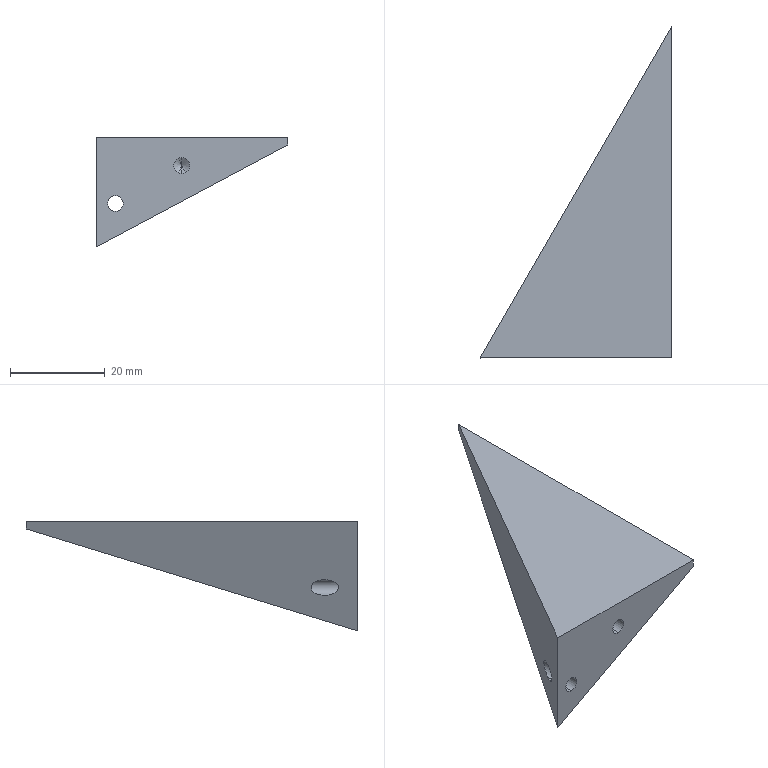Part | STEP file | GLSJ-10-26_default | 1 solid | 11 faces | box 40.415 x 70 x 23.157 mm | volume 12343 mm3 | plane 5 | cylinder 4 | cone 2 | commonest cylinder face diameters 3.3 x4
STEP:
#1=CARTESIAN_POINT('',(0.,0.,0.));
#2=DIRECTION('',(0.,0.,1.));
#3=DIRECTION('',(1.,0.,0.));
#4=AXIS2_PLACEMENT_3D('',#1,#2,#3);
#5=CARTESIAN_POINT('',(-36.372,7.003,8.35));
#6=VERTEX_POINT('',#5);
#7=CARTESIAN_POINT('',(-36.372,0.,8.35));
#8=VERTEX_POINT('',#7);
#9=CARTESIAN_POINT('',(-36.372,0.,8.35));
#10=DIRECTION('',(0.,-1.,0.));
#11=VECTOR('',#10,1.);
#12=LINE('',#9,#11);
#13=CARTESIAN_POINT('',(-36.372,0.,10.));
#14=DIRECTION('',(0.,-1.,0.));
#15=DIRECTION('',(0.,0.,-1.));
#16=AXIS2_PLACEMENT_3D('',#13,#14,#15);
#17=CYLINDRICAL_SURFACE('',#16,1.65);
#18=CARTESIAN_POINT('',(6.283,0.));
#19=DIRECTION('',(0.,1.));
#20=VECTOR('',#19,1.);
#21=LINE('',#18,#20);
#22=(GEOMETRIC_REPRESENTATION_CONTEXT(2)PARAMETRIC_REPRESENTATION_CONTEXT()REPRESENTATION_CONTEXT('',''));
#23=DEFINITIONAL_REPRESENTATION('',(#21),#22);
#24=PCURVE('',#17,#23);
#25=CARTESIAN_POINT('',(-36.372,0.,10.));
#26=DIRECTION('',(0.,-1.,0.));
#27=DIRECTION('',(0.,0.,-1.));
#28=AXIS2_PLACEMENT_3D('',#25,#26,#27);
#29=CYLINDRICAL_SURFACE('',#28,1.65);
#30=CARTESIAN_POINT('',(0.,0.));
#31=DIRECTION('',(0.,1.));
#32=VECTOR('',#31,1.);
#33=LINE('',#30,#32);
#34=(GEOMETRIC_REPRESENTATION_CONTEXT(2)PARAMETRIC_REPRESENTATION_CONTEXT()REPRESENTATION_CONTEXT('',''));
#35=DEFINITIONAL_REPRESENTATION('',(#33),#34);
#36=PCURVE('',#29,#35);
#37=SURFACE_CURVE('',#12,(#24,#36),.PCURVE_S1.);
#38=EDGE_CURVE('',#6,#8,#37,.T.);
#39=ORIENTED_EDGE('',*,*,#38,.T.);
#40=CARTESIAN_POINT('',(-36.372,0.,11.65));
#41=VERTEX_POINT('',#40);
#42=CARTESIAN_POINT('',(-36.372,0.,10.));
#43=DIRECTION('',(0.,-1.,0.));
#44=DIRECTION('',(0.,0.,-1.));
#45=AXIS2_PLACEMENT_3D('',#42,#43,#44);
#46=CIRCLE('',#45,1.65);
#47=CARTESIAN_POINT('',(0.,0.));
#48=DIRECTION('',(1.,0.));
#49=VECTOR('',#48,1.);
#50=LINE('',#47,#49);
#51=(GEOMETRIC_REPRESENTATION_CONTEXT(2)PARAMETRIC_REPRESENTATION_CONTEXT()REPRESENTATION_CONTEXT('',''));
#52=DEFINITIONAL_REPRESENTATION('',(#50),#51);
#53=PCURVE('',#17,#52);
#54=CARTESIAN_POINT('',(-40.415,0.,24.));
#55=DIRECTION('',(0.,1.,0.));
#56=DIRECTION('',(-1.,0.,0.));
#57=AXIS2_PLACEMENT_3D('',#54,#55,#56);
#58=PLANE('',#57);
#59=CARTESIAN_POINT('',(-4.043,-15.65));
#60=CARTESIAN_POINT('',(-6.901,-15.65));
#61=CARTESIAN_POINT('',(-5.472,-13.175));
#62=CARTESIAN_POINT('',(-4.043,-10.7));
#63=CARTESIAN_POINT('',(-2.614,-13.175));
#64=CARTESIAN_POINT('',(-1.185,-15.65));
#65=CARTESIAN_POINT('',(-4.043,-15.65));
#66=(BOUNDED_CURVE()B_SPLINE_CURVE(2,(#59,#60,#61,#62,#63,#64,#65),.UNSPECIFIED.,.T.,.F.)B_SPLINE_CURVE_WITH_KNOTS((1,2,2,2,2,1),(-2.094,0.,2.094,4.189,6.283,8.378),.UNSPECIFIED.)CURVE()GEOMETRIC_REPRESENTATION_ITEM()RATIONAL_B_SPLINE_CURVE((1.,0.5,1.,0.5,1.,0.5,1.))REPRESENTATION_ITEM(''));
#67=(GEOMETRIC_REPRESENTATION_CONTEXT(2)PARAMETRIC_REPRESENTATION_CONTEXT()REPRESENTATION_CONTEXT('',''));
#68=DEFINITIONAL_REPRESENTATION('',(#66),#67);
#69=PCURVE('',#58,#68);
#70=SURFACE_CURVE('',#46,(#53,#69),.PCURVE_S1.);
#71=EDGE_CURVE('',#41,#8,#70,.T.);
#72=ORIENTED_EDGE('',*,*,#71,.F.);
#73=CARTESIAN_POINT('',(-36.372,7.003,11.65));
#74=VERTEX_POINT('',#73);
#75=CARTESIAN_POINT('',(-36.372,0.,11.65));
#76=DIRECTION('',(0.,-1.,0.));
#77=VECTOR('',#76,1.);
#78=LINE('',#75,#77);
#79=CARTESIAN_POINT('',(3.142,0.));
#80=DIRECTION('',(0.,1.));
#81=VECTOR('',#80,1.);
#82=LINE('',#79,#81);
#83=(GEOMETRIC_REPRESENTATION_CONTEXT(2)PARAMETRIC_REPRESENTATION_CONTEXT()REPRESENTATION_CONTEXT('',''));
#84=DEFINITIONAL_REPRESENTATION('',(#82),#83);
#85=PCURVE('',#17,#84);
#86=CARTESIAN_POINT('',(3.142,0.));
#87=DIRECTION('',(0.,1.));
#88=VECTOR('',#87,1.);
#89=LINE('',#86,#88);
#90=(GEOMETRIC_REPRESENTATION_CONTEXT(2)PARAMETRIC_REPRESENTATION_CONTEXT()REPRESENTATION_CONTEXT('',''));
#91=DEFINITIONAL_REPRESENTATION('',(#89),#90);
#92=PCURVE('',#29,#91);
#93=SURFACE_CURVE('',#78,(#85,#92),.PCURVE_S1.);
#94=EDGE_CURVE('',#74,#41,#93,.T.);
#95=ORIENTED_EDGE('',*,*,#94,.F.);
#96=CARTESIAN_POINT('',(-36.372,7.003,11.65));
#97=CARTESIAN_POINT('',(-39.672,1.287,11.65));
#98=CARTESIAN_POINT('',(-39.672,1.287,8.35));
#99=CARTESIAN_POINT('',(-36.372,7.003,8.35));
#100=(BOUNDED_CURVE()B_SPLINE_CURVE(3,(#96,#97,#98,#99),.UNSPECIFIED.,.F.,.F.)B_SPLINE_CURVE_WITH_KNOTS((4,4),(4.712,7.854),.PIECEWISE_BEZIER_KNOTS.)CURVE()GEOMETRIC_REPRESENTATION_ITEM()RATIONAL_B_SPLINE_CURVE((1.,0.3333,0.3333,1.))REPRESENTATION_ITEM(''));
#101=CARTESIAN_POINT('',(3.142,-7.003));
#102=CARTESIAN_POINT('',(3.172,-6.916));
#103=CARTESIAN_POINT('',(3.235,-6.735));
#104=CARTESIAN_POINT('',(3.339,-6.44));
#105=CARTESIAN_POINT('',(3.453,-6.125));
#106=CARTESIAN_POINT('',(3.577,-5.793));
#107=CARTESIAN_POINT('',(3.712,-5.455));
#108=CARTESIAN_POINT('',(3.857,-5.12));
#109=CARTESIAN_POINT('',(4.013,-4.806));
#110=CARTESIAN_POINT('',(4.179,-4.531));
#111=CARTESIAN_POINT('',(4.352,-4.315));
#112=CARTESIAN_POINT('',(4.531,-4.176));
#113=CARTESIAN_POINT('',(4.712,-4.129));
#114=CARTESIAN_POINT('',(4.894,-4.176));
#115=CARTESIAN_POINT('',(5.073,-4.315));
#116=CARTESIAN_POINT('',(5.246,-4.531));
#117=CARTESIAN_POINT('',(5.412,-4.806));
#118=CARTESIAN_POINT('',(5.567,-5.12));
#119=CARTESIAN_POINT('',(5.713,-5.455));
#120=CARTESIAN_POINT('',(5.848,-5.793));
#121=CARTESIAN_POINT('',(5.972,-6.125));
#122=CARTESIAN_POINT('',(6.085,-6.44));
#123=CARTESIAN_POINT('',(6.19,-6.735));
#124=CARTESIAN_POINT('',(6.253,-6.916));
#125=CARTESIAN_POINT('',(6.283,-7.003));
#126=B_SPLINE_CURVE_WITH_KNOTS('',3,(#101,#102,#103,#104,#105,#106,#107,#108,#109,#110,#111,#112,#113,#114,#115,#116,#117,#118,#119,#120,#121,#122,#123,#124,#125),.UNSPECIFIED.,.F.,.F.,(4,1,1,1,1,1,1,1,1,1,1,1,1,1,1,1,1,1,1,1,1,1,4),(4.712,4.855,4.998,5.141,5.284,5.426,5.569,5.712,5.855,5.998,6.14,6.283,6.426,6.569,6.712,6.854,6.997,7.14,7.283,7.426,7.568,7.711,7.854),.QUASI_UNIFORM_KNOTS.);
#127=(GEOMETRIC_REPRESENTATION_CONTEXT(2)PARAMETRIC_REPRESENTATION_CONTEXT()REPRESENTATION_CONTEXT('',''));
#128=DEFINITIONAL_REPRESENTATION('',(#126),#127);
#129=PCURVE('',#17,#128);
#130=CARTESIAN_POINT('',(0.,70.,24.));
#131=DIRECTION('',(0.866,-0.5,0.));
#132=DIRECTION('',(0.5,0.866,0.));
#133=AXIS2_PLACEMENT_3D('',#130,#131,#132);
#134=PLANE('',#133);
#135=CARTESIAN_POINT('',(-72.743,-12.35));
#136=CARTESIAN_POINT('',(-79.343,-12.35));
#137=CARTESIAN_POINT('',(-79.343,-15.65));
#138=CARTESIAN_POINT('',(-72.743,-15.65));
#139=(BOUNDED_CURVE()B_SPLINE_CURVE(3,(#135,#136,#137,#138),.UNSPECIFIED.,.F.,.F.)B_SPLINE_CURVE_WITH_KNOTS((4,4),(4.712,7.854),.PIECEWISE_BEZIER_KNOTS.)CURVE()GEOMETRIC_REPRESENTATION_ITEM()RATIONAL_B_SPLINE_CURVE((1.,0.3333,0.3333,1.))REPRESENTATION_ITEM(''));
#140=(GEOMETRIC_REPRESENTATION_CONTEXT(2)PARAMETRIC_REPRESENTATION_CONTEXT()REPRESENTATION_CONTEXT('',''));
#141=DEFINITIONAL_REPRESENTATION('',(#139),#140);
#142=PCURVE('',#134,#141);
#143=SURFACE_CURVE('',#100,(#129,#142),.PCURVE_S1.);
#144=EDGE_CURVE('',#74,#6,#143,.T.);
#145=ORIENTED_EDGE('',*,*,#144,.T.);
#146=EDGE_LOOP('',(#39,#72,#95,#145));
#147=FACE_BOUND('',#146,.F.);
#148=ADVANCED_FACE('',(#147),#17,.F.);
#149=CARTESIAN_POINT('',(-22.372,10.1,16.35));
#150=VERTEX_POINT('',#149);
#151=CARTESIAN_POINT('',(-22.372,0.,16.35));
#152=VERTEX_POINT('',#151);
#153=CARTESIAN_POINT('',(-22.372,0.,16.35));
#154=DIRECTION('',(0.,-1.,0.));
#155=VECTOR('',#154,1.);
#156=LINE('',#153,#155);
#157=CARTESIAN_POINT('',(-22.372,0.,18.));
#158=DIRECTION('',(0.,-1.,0.));
#159=DIRECTION('',(0.,0.,-1.));
#160=AXIS2_PLACEMENT_3D('',#157,#158,#159);
#161=CYLINDRICAL_SURFACE('',#160,1.65);
#162=CARTESIAN_POINT('',(6.283,0.));
#163=DIRECTION('',(0.,1.));
#164=VECTOR('',#163,1.);
#165=LINE('',#162,#164);
#166=(GEOMETRIC_REPRESENTATION_CONTEXT(2)PARAMETRIC_REPRESENTATION_CONTEXT()REPRESENTATION_CONTEXT('',''));
#167=DEFINITIONAL_REPRESENTATION('',(#165),#166);
#168=PCURVE('',#161,#167);
#169=CARTESIAN_POINT('',(-22.372,0.,18.));
#170=DIRECTION('',(0.,-1.,0.));
#171=DIRECTION('',(0.,0.,-1.));
#172=AXIS2_PLACEMENT_3D('',#169,#170,#171);
#173=CYLINDRICAL_SURFACE('',#172,1.65);
#174=CARTESIAN_POINT('',(0.,0.));
#175=DIRECTION('',(0.,1.));
#176=VECTOR('',#175,1.);
#177=LINE('',#174,#176);
#178=(GEOMETRIC_REPRESENTATION_CONTEXT(2)PARAMETRIC_REPRESENTATION_CONTEXT()REPRESENTATION_CONTEXT('',''));
#179=DEFINITIONAL_REPRESENTATION('',(#177),#178);
#180=PCURVE('',#173,#179);
#181=SURFACE_CURVE('',#156,(#168,#180),.PCURVE_S1.);
#182=EDGE_CURVE('',#150,#152,#181,.T.);
#183=ORIENTED_EDGE('',*,*,#182,.T.);
#184=CARTESIAN_POINT('',(-22.372,0.,19.65));
#185=VERTEX_POINT('',#184);
#186=CARTESIAN_POINT('',(-22.372,0.,18.));
#187=DIRECTION('',(0.,-1.,0.));
#188=DIRECTION('',(0.,0.,-1.));
#189=AXIS2_PLACEMENT_3D('',#186,#187,#188);
#190=CIRCLE('',#189,1.65);
#191=CARTESIAN_POINT('',(0.,0.));
#192=DIRECTION('',(1.,0.));
#193=VECTOR('',#192,1.);
#194=LINE('',#191,#193);
#195=(GEOMETRIC_REPRESENTATION_CONTEXT(2)PARAMETRIC_REPRESENTATION_CONTEXT()REPRESENTATION_CONTEXT('',''));
#196=DEFINITIONAL_REPRESENTATION('',(#194),#195);
#197=PCURVE('',#161,#196);
#198=CARTESIAN_POINT('',(-18.043,-7.65));
#199=CARTESIAN_POINT('',(-20.901,-7.65));
#200=CARTESIAN_POINT('',(-19.472,-5.175));
#201=CARTESIAN_POINT('',(-18.043,-2.7));
#202=CARTESIAN_POINT('',(-16.614,-5.175));
#203=CARTESIAN_POINT('',(-15.185,-7.65));
#204=CARTESIAN_POINT('',(-18.043,-7.65));
#205=(BOUNDED_CURVE()B_SPLINE_CURVE(2,(#198,#199,#200,#201,#202,#203,#204),.UNSPECIFIED.,.T.,.F.)B_SPLINE_CURVE_WITH_KNOTS((1,2,2,2,2,1),(-2.094,0.,2.094,4.189,6.283,8.378),.UNSPECIFIED.)CURVE()GEOMETRIC_REPRESENTATION_ITEM()RATIONAL_B_SPLINE_CURVE((1.,0.5,1.,0.5,1.,0.5,1.))REPRESENTATION_ITEM(''));
#206=(GEOMETRIC_REPRESENTATION_CONTEXT(2)PARAMETRIC_REPRESENTATION_CONTEXT()REPRESENTATION_CONTEXT('',''));
#207=DEFINITIONAL_REPRESENTATION('',(#205),#206);
#208=PCURVE('',#58,#207);
#209=SURFACE_CURVE('',#190,(#197,#208),.PCURVE_S1.);
#210=EDGE_CURVE('',#185,#152,#209,.T.);
#211=ORIENTED_EDGE('',*,*,#210,.F.);
#212=CARTESIAN_POINT('',(-22.372,10.1,19.65));
#213=VERTEX_POINT('',#212);
#214=CARTESIAN_POINT('',(-22.372,0.,19.65));
#215=DIRECTION('',(0.,-1.,0.));
#216=VECTOR('',#215,1.);
#217=LINE('',#214,#216);
#218=CARTESIAN_POINT('',(3.142,0.));
#219=DIRECTION('',(0.,1.));
#220=VECTOR('',#219,1.);
#221=LINE('',#218,#220);
#222=(GEOMETRIC_REPRESENTATION_CONTEXT(2)PARAMETRIC_REPRESENTATION_CONTEXT()REPRESENTATION_CONTEXT('',''));
#223=DEFINITIONAL_REPRESENTATION('',(#221),#222);
#224=PCURVE('',#161,#223);
#225=CARTESIAN_POINT('',(3.142,0.));
#226=DIRECTION('',(0.,1.));
#227=VECTOR('',#226,1.);
#228=LINE('',#225,#227);
#229=(GEOMETRIC_REPRESENTATION_CONTEXT(2)PARAMETRIC_REPRESENTATION_CONTEXT()REPRESENTATION_CONTEXT('',''));
#230=DEFINITIONAL_REPRESENTATION('',(#228),#229);
#231=PCURVE('',#173,#230);
#232=SURFACE_CURVE('',#217,(#224,#231),.PCURVE_S1.);
#233=EDGE_CURVE('',#213,#185,#232,.T.);
#234=ORIENTED_EDGE('',*,*,#233,.F.);
#235=CARTESIAN_POINT('',(-22.372,10.1,18.));
#236=DIRECTION('',(0.,-1.,0.));
#237=DIRECTION('',(0.,0.,-1.));
#238=AXIS2_PLACEMENT_3D('',#235,#236,#237);
#239=CIRCLE('',#238,1.65);
#240=CARTESIAN_POINT('',(0.,-10.1));
#241=DIRECTION('',(1.,0.));
#242=VECTOR('',#241,1.);
#243=LINE('',#240,#242);
#244=(GEOMETRIC_REPRESENTATION_CONTEXT(2)PARAMETRIC_REPRESENTATION_CONTEXT()REPRESENTATION_CONTEXT('',''));
#245=DEFINITIONAL_REPRESENTATION('',(#243),#244);
#246=PCURVE('',#161,#245);
#247=CARTESIAN_POINT('',(-22.372,10.1,18.));
#248=DIRECTION('',(0.,-1.,0.));
#249=DIRECTION('',(0.,0.,-1.));
#250=AXIS2_PLACEMENT_3D('',#247,#248,#249);
#251=CONICAL_SURFACE('',#250,1.65,1.03);
#252=CARTESIAN_POINT('',(0.,0.));
#253=DIRECTION('',(1.,0.));
#254=VECTOR('',#253,1.);
#255=LINE('',#252,#254);
#256=(GEOMETRIC_REPRESENTATION_CONTEXT(2)PARAMETRIC_REPRESENTATION_CONTEXT()REPRESENTATION_CONTEXT('',''));
#257=DEFINITIONAL_REPRESENTATION('',(#255),#256);
#258=PCURVE('',#251,#257);
#259=SURFACE_CURVE('',#239,(#246,#258),.PCURVE_S1.);
#260=EDGE_CURVE('',#213,#150,#259,.T.);
#261=ORIENTED_EDGE('',*,*,#260,.T.);
#262=EDGE_LOOP('',(#183,#211,#234,#261));
#263=FACE_BOUND('',#262,.F.);
#264=ADVANCED_FACE('',(#263),#161,.F.);
#265=ORIENTED_EDGE('',*,*,#260,.F.);
#266=CARTESIAN_POINT('',(-22.372,11.091,18.));
#267=VERTEX_POINT('',#266);
#268=CARTESIAN_POINT('',(-22.372,10.1,19.65));
#269=DIRECTION('',(0.,-0.515,0.8572));
#270=VECTOR('',#269,1.);
#271=LINE('',#268,#270);
#272=CARTESIAN_POINT('',(3.142,-0.9914));
#273=CARTESIAN_POINT('',(3.142,-0.9764));
#274=CARTESIAN_POINT('',(3.142,-0.9464));
#275=CARTESIAN_POINT('',(3.142,-0.9013));
#276=CARTESIAN_POINT('',(3.142,-0.8562));
#277=CARTESIAN_POINT('',(3.142,-0.8112));
#278=CARTESIAN_POINT('',(3.142,-0.7661));
#279=CARTESIAN_POINT('',(3.142,-0.721));
#280=CARTESIAN_POINT('',(3.142,-0.676));
#281=CARTESIAN_POINT('',(3.142,-0.6309));
#282=CARTESIAN_POINT('',(3.142,-0.5858));
#283=CARTESIAN_POINT('',(3.142,-0.5408));
#284=CARTESIAN_POINT('',(3.142,-0.4957));
#285=CARTESIAN_POINT('',(3.142,-0.4506));
#286=CARTESIAN_POINT('',(3.142,-0.4056));
#287=CARTESIAN_POINT('',(3.142,-0.3605));
#288=CARTESIAN_POINT('',(3.142,-0.3155));
#289=CARTESIAN_POINT('',(3.142,-0.2704));
#290=CARTESIAN_POINT('',(3.142,-0.2253));
#291=CARTESIAN_POINT('',(3.142,-0.1803));
#292=CARTESIAN_POINT('',(3.142,-0.1352));
#293=CARTESIAN_POINT('',(3.142,-0.09013));
#294=CARTESIAN_POINT('',(3.142,-0.04506));
#295=CARTESIAN_POINT('',(3.142,-0.01502));
#296=CARTESIAN_POINT('',(3.142,0.));
#297=B_SPLINE_CURVE_WITH_KNOTS('',3,(#272,#273,#274,#275,#276,#277,#278,#279,#280,#281,#282,#283,#284,#285,#286,#287,#288,#289,#290,#291,#292,#293,#294,#295,#296),.UNSPECIFIED.,.F.,.F.,(4,1,1,1,1,1,1,1,1,1,1,1,1,1,1,1,1,1,1,1,1,1,4),(-1.925,-1.837,-1.75,-1.662,-1.575,-1.487,-1.4,-1.312,-1.225,-1.137,-1.05,-0.9625,-0.875,-0.7875,-0.7,-0.6125,-0.525,-0.4375,-0.35,-0.2625,-0.175,-0.0875,0.),.QUASI_UNIFORM_KNOTS.);
#298=(GEOMETRIC_REPRESENTATION_CONTEXT(2)PARAMETRIC_REPRESENTATION_CONTEXT()REPRESENTATION_CONTEXT('',''));
#299=DEFINITIONAL_REPRESENTATION('',(#297),#298);
#300=PCURVE('',#251,#299);
#301=CARTESIAN_POINT('',(-22.372,10.1,18.));
#302=DIRECTION('',(0.,-1.,0.));
#303=DIRECTION('',(0.,0.,-1.));
#304=AXIS2_PLACEMENT_3D('',#301,#302,#303);
#305=CONICAL_SURFACE('',#304,1.65,1.03);
#306=CARTESIAN_POINT('',(3.142,-0.9914));
#307=CARTESIAN_POINT('',(3.142,-0.9764));
#308=CARTESIAN_POINT('',(3.142,-0.9464));
#309=CARTESIAN_POINT('',(3.142,-0.9013));
#310=CARTESIAN_POINT('',(3.142,-0.8562));
#311=CARTESIAN_POINT('',(3.142,-0.8112));
#312=CARTESIAN_POINT('',(3.142,-0.7661));
#313=CARTESIAN_POINT('',(3.142,-0.721));
#314=CARTESIAN_POINT('',(3.142,-0.676));
#315=CARTESIAN_POINT('',(3.142,-0.6309));
#316=CARTESIAN_POINT('',(3.142,-0.5858));
#317=CARTESIAN_POINT('',(3.142,-0.5408));
#318=CARTESIAN_POINT('',(3.142,-0.4957));
#319=CARTESIAN_POINT('',(3.142,-0.4506));
#320=CARTESIAN_POINT('',(3.142,-0.4056));
#321=CARTESIAN_POINT('',(3.142,-0.3605));
#322=CARTESIAN_POINT('',(3.142,-0.3155));
#323=CARTESIAN_POINT('',(3.142,-0.2704));
#324=CARTESIAN_POINT('',(3.142,-0.2253));
#325=CARTESIAN_POINT('',(3.142,-0.1803));
#326=CARTESIAN_POINT('',(3.142,-0.1352));
#327=CARTESIAN_POINT('',(3.142,-0.09013));
#328=CARTESIAN_POINT('',(3.142,-0.04506));
#329=CARTESIAN_POINT('',(3.142,-0.01502));
#330=CARTESIAN_POINT('',(3.142,0.));
#331=B_SPLINE_CURVE_WITH_KNOTS('',3,(#306,#307,#308,#309,#310,#311,#312,#313,#314,#315,#316,#317,#318,#319,#320,#321,#322,#323,#324,#325,#326,#327,#328,#329,#330),.UNSPECIFIED.,.F.,.F.,(4,1,1,1,1,1,1,1,1,1,1,1,1,1,1,1,1,1,1,1,1,1,4),(-1.925,-1.837,-1.75,-1.662,-1.575,-1.487,-1.4,-1.312,-1.225,-1.137,-1.05,-0.9625,-0.875,-0.7875,-0.7,-0.6125,-0.525,-0.4375,-0.35,-0.2625,-0.175,-0.0875,0.),.QUASI_UNIFORM_KNOTS.);
#332=(GEOMETRIC_REPRESENTATION_CONTEXT(2)PARAMETRIC_REPRESENTATION_CONTEXT()REPRESENTATION_CONTEXT('',''));
#333=DEFINITIONAL_REPRESENTATION('',(#331),#332);
#334=PCURVE('',#305,#333);
#335=SURFACE_CURVE('',#271,(#300,#334),.PCURVE_S1.);
#336=EDGE_CURVE('',#267,#213,#335,.T.);
#337=ORIENTED_EDGE('',*,*,#336,.F.);
#338=CARTESIAN_POINT('',(-22.372,10.1,16.35));
#339=DIRECTION('',(0.,-0.515,-0.8572));
#340=VECTOR('',#339,1.);
#341=LINE('',#338,#340);
#342=CARTESIAN_POINT('',(6.283,0.));
#343=DIRECTION('',(0.,1.));
#344=VECTOR('',#343,1.);
#345=LINE('',#342,#344);
#346=(GEOMETRIC_REPRESENTATION_CONTEXT(2)PARAMETRIC_REPRESENTATION_CONTEXT()REPRESENTATION_CONTEXT('',''));
#347=DEFINITIONAL_REPRESENTATION('',(#345),#346);
#348=PCURVE('',#251,#347);
#349=CARTESIAN_POINT('',(0.,0.));
#350=DIRECTION('',(0.,1.));
#351=VECTOR('',#350,1.);
#352=LINE('',#349,#351);
#353=(GEOMETRIC_REPRESENTATION_CONTEXT(2)PARAMETRIC_REPRESENTATION_CONTEXT()REPRESENTATION_CONTEXT('',''));
#354=DEFINITIONAL_REPRESENTATION('',(#352),#353);
#355=PCURVE('',#305,#354);
#356=SURFACE_CURVE('',#341,(#348,#355),.PCURVE_S1.);
#357=EDGE_CURVE('',#267,#150,#356,.T.);
#358=ORIENTED_EDGE('',*,*,#357,.T.);
#359=EDGE_LOOP('',(#265,#337,#358));
#360=FACE_BOUND('',#359,.F.);
#361=ADVANCED_FACE('',(#360),#251,.F.);
#362=CARTESIAN_POINT('',(-36.372,0.,10.));
#363=DIRECTION('',(0.,-1.,0.));
#364=DIRECTION('',(0.,0.,-1.));
#365=AXIS2_PLACEMENT_3D('',#362,#363,#364);
#366=CIRCLE('',#365,1.65);
#367=CARTESIAN_POINT('',(-4.043,-15.65));
#368=CARTESIAN_POINT('',(-6.901,-15.65));
#369=CARTESIAN_POINT('',(-5.472,-13.175));
#370=CARTESIAN_POINT('',(-4.043,-10.7));
#371=CARTESIAN_POINT('',(-2.614,-13.175));
#372=CARTESIAN_POINT('',(-1.185,-15.65));
#373=CARTESIAN_POINT('',(-4.043,-15.65));
#374=(BOUNDED_CURVE()B_SPLINE_CURVE(2,(#367,#368,#369,#370,#371,#372,#373),.UNSPECIFIED.,.T.,.F.)B_SPLINE_CURVE_WITH_KNOTS((1,2,2,2,2,1),(-2.094,0.,2.094,4.189,6.283,8.378),.UNSPECIFIED.)CURVE()GEOMETRIC_REPRESENTATION_ITEM()RATIONAL_B_SPLINE_CURVE((1.,0.5,1.,0.5,1.,0.5,1.))REPRESENTATION_ITEM(''));
#375=(GEOMETRIC_REPRESENTATION_CONTEXT(2)PARAMETRIC_REPRESENTATION_CONTEXT()REPRESENTATION_CONTEXT('',''));
#376=DEFINITIONAL_REPRESENTATION('',(#374),#375);
#377=PCURVE('',#58,#376);
#378=CARTESIAN_POINT('',(0.,0.));
#379=DIRECTION('',(1.,0.));
#380=VECTOR('',#379,1.);
#381=LINE('',#378,#380);
#382=(GEOMETRIC_REPRESENTATION_CONTEXT(2)PARAMETRIC_REPRESENTATION_CONTEXT()REPRESENTATION_CONTEXT('',''));
#383=DEFINITIONAL_REPRESENTATION('',(#381),#382);
#384=PCURVE('',#29,#383);
#385=SURFACE_CURVE('',#366,(#377,#384),.PCURVE_S1.);
#386=EDGE_CURVE('',#8,#41,#385,.T.);
#387=ORIENTED_EDGE('',*,*,#386,.F.);
#388=ORIENTED_EDGE('',*,*,#71,.F.);
#389=EDGE_LOOP('',(#387,#388));
#390=FACE_BOUND('',#389,.T.);
#391=CARTESIAN_POINT('',(-22.372,0.,18.));
#392=DIRECTION('',(0.,-1.,0.));
#393=DIRECTION('',(0.,0.,-1.));
#394=AXIS2_PLACEMENT_3D('',#391,#392,#393);
#395=CIRCLE('',#394,1.65);
#396=CARTESIAN_POINT('',(-18.043,-7.65));
#397=CARTESIAN_POINT('',(-20.901,-7.65));
#398=CARTESIAN_POINT('',(-19.472,-5.175));
#399=CARTESIAN_POINT('',(-18.043,-2.7));
#400=CARTESIAN_POINT('',(-16.614,-5.175));
#401=CARTESIAN_POINT('',(-15.185,-7.65));
#402=CARTESIAN_POINT('',(-18.043,-7.65));
#403=(BOUNDED_CURVE()B_SPLINE_CURVE(2,(#396,#397,#398,#399,#400,#401,#402),.UNSPECIFIED.,.T.,.F.)B_SPLINE_CURVE_WITH_KNOTS((1,2,2,2,2,1),(-2.094,0.,2.094,4.189,6.283,8.378),.UNSPECIFIED.)CURVE()GEOMETRIC_REPRESENTATION_ITEM()RATIONAL_B_SPLINE_CURVE((1.,0.5,1.,0.5,1.,0.5,1.))REPRESENTATION_ITEM(''));
#404=(GEOMETRIC_REPRESENTATION_CONTEXT(2)PARAMETRIC_REPRESENTATION_CONTEXT()REPRESENTATION_CONTEXT('',''));
#405=DEFINITIONAL_REPRESENTATION('',(#403),#404);
#406=PCURVE('',#58,#405);
#407=CARTESIAN_POINT('',(0.,0.));
#408=DIRECTION('',(1.,0.));
#409=VECTOR('',#408,1.);
#410=LINE('',#407,#409);
#411=(GEOMETRIC_REPRESENTATION_CONTEXT(2)PARAMETRIC_REPRESENTATION_CONTEXT()REPRESENTATION_CONTEXT('',''));
#412=DEFINITIONAL_REPRESENTATION('',(#410),#411);
#413=PCURVE('',#173,#412);
#414=SURFACE_CURVE('',#395,(#406,#413),.PCURVE_S1.);
#415=EDGE_CURVE('',#152,#185,#414,.T.);
#416=ORIENTED_EDGE('',*,*,#415,.F.);
#417=ORIENTED_EDGE('',*,*,#210,.F.);
#418=EDGE_LOOP('',(#416,#417));
#419=FACE_BOUND('',#418,.T.);
#420=CARTESIAN_POINT('',(-40.415,0.,24.));
#421=VERTEX_POINT('',#420);
#422=CARTESIAN_POINT('',(-40.415,0.,0.843));
#423=VERTEX_POINT('',#422);
#424=CARTESIAN_POINT('',(-40.415,0.,24.));
#425=DIRECTION('',(0.,0.,-1.));
#426=VECTOR('',#425,1.);
#427=LINE('',#424,#426);
#428=CARTESIAN_POINT('',(0.,0.));
#429=DIRECTION('',(0.,-1.));
#430=VECTOR('',#429,1.);
#431=LINE('',#428,#430);
#432=(GEOMETRIC_REPRESENTATION_CONTEXT(2)PARAMETRIC_REPRESENTATION_CONTEXT()REPRESENTATION_CONTEXT('',''));
#433=DEFINITIONAL_REPRESENTATION('',(#431),#432);
#434=PCURVE('',#58,#433);
#435=CARTESIAN_POINT('',(-80.829,0.));
#436=DIRECTION('',(0.,-1.));
#437=VECTOR('',#436,1.);
#438=LINE('',#435,#437);
#439=(GEOMETRIC_REPRESENTATION_CONTEXT(2)PARAMETRIC_REPRESENTATION_CONTEXT()REPRESENTATION_CONTEXT('',''));
#440=DEFINITIONAL_REPRESENTATION('',(#438),#439);
#441=PCURVE('',#134,#440);
#442=SURFACE_CURVE('',#427,(#434,#441),.PCURVE_S1.);
#443=EDGE_CURVE('',#421,#423,#442,.T.);
#444=ORIENTED_EDGE('',*,*,#443,.T.);
#445=CARTESIAN_POINT('',(0.,0.,22.332));
#446=VERTEX_POINT('',#445);
#447=CARTESIAN_POINT('',(0.,0.,22.332));
#448=DIRECTION('',(0.8829,0.,0.4695));
#449=VECTOR('',#448,1.);
#450=LINE('',#447,#449);
#451=CARTESIAN_POINT('',(-40.415,-1.668));
#452=DIRECTION('',(-0.8829,0.4695));
#453=VECTOR('',#452,1.);
#454=LINE('',#451,#453);
#455=(GEOMETRIC_REPRESENTATION_CONTEXT(2)PARAMETRIC_REPRESENTATION_CONTEXT()REPRESENTATION_CONTEXT('',''));
#456=DEFINITIONAL_REPRESENTATION('',(#454),#455);
#457=PCURVE('',#58,#456);
#458=CARTESIAN_POINT('',(0.,0.,22.332));
#459=DIRECTION('',(-0.4695,0.,0.8829));
#460=DIRECTION('',(0.,1.,0.));
#461=AXIS2_PLACEMENT_3D('',#458,#459,#460);
#462=PLANE('',#461);
#463=CARTESIAN_POINT('',(0.,0.));
#464=DIRECTION('',(0.,-1.));
#465=VECTOR('',#464,1.);
#466=LINE('',#463,#465);
#467=(GEOMETRIC_REPRESENTATION_CONTEXT(2)PARAMETRIC_REPRESENTATION_CONTEXT()REPRESENTATION_CONTEXT('',''));
#468=DEFINITIONAL_REPRESENTATION('',(#466),#467);
#469=PCURVE('',#462,#468);
#470=SURFACE_CURVE('',#450,(#457,#469),.PCURVE_S1.);
#471=EDGE_CURVE('',#423,#446,#470,.T.);
#472=ORIENTED_EDGE('',*,*,#471,.T.);
#473=CARTESIAN_POINT('',(0.,0.,24.));
#474=VERTEX_POINT('',#473);
#475=CARTESIAN_POINT('',(0.,0.,24.));
#476=DIRECTION('',(0.,0.,-1.));
#477=VECTOR('',#476,1.);
#478=LINE('',#475,#477);
#479=CARTESIAN_POINT('',(-40.415,0.));
#480=DIRECTION('',(0.,-1.));
#481=VECTOR('',#480,1.);
#482=LINE('',#479,#481);
#483=(GEOMETRIC_REPRESENTATION_CONTEXT(2)PARAMETRIC_REPRESENTATION_CONTEXT()REPRESENTATION_CONTEXT('',''));
#484=DEFINITIONAL_REPRESENTATION('',(#482),#483);
#485=PCURVE('',#58,#484);
#486=CARTESIAN_POINT('',(0.,0.,24.));
#487=DIRECTION('',(-1.,0.,0.));
#488=DIRECTION('',(0.,0.,1.));
#489=AXIS2_PLACEMENT_3D('',#486,#487,#488);
#490=PLANE('',#489);
#491=CARTESIAN_POINT('',(0.,0.));
#492=DIRECTION('',(-1.,0.));
#493=VECTOR('',#492,1.);
#494=LINE('',#491,#493);
#495=(GEOMETRIC_REPRESENTATION_CONTEXT(2)PARAMETRIC_REPRESENTATION_CONTEXT()REPRESENTATION_CONTEXT('',''));
#496=DEFINITIONAL_REPRESENTATION('',(#494),#495);
#497=PCURVE('',#490,#496);
#498=SURFACE_CURVE('',#478,(#485,#497),.PCURVE_S1.);
#499=EDGE_CURVE('',#474,#446,#498,.T.);
#500=ORIENTED_EDGE('',*,*,#499,.F.);
#501=CARTESIAN_POINT('',(-40.415,0.,24.));
#502=DIRECTION('',(1.,0.,0.));
#503=VECTOR('',#502,1.);
#504=LINE('',#501,#503);
#505=CARTESIAN_POINT('',(0.,0.));
#506=DIRECTION('',(-1.,0.));
#507=VECTOR('',#506,1.);
#508=LINE('',#505,#507);
#509=(GEOMETRIC_REPRESENTATION_CONTEXT(2)PARAMETRIC_REPRESENTATION_CONTEXT()REPRESENTATION_CONTEXT('',''));
#510=DEFINITIONAL_REPRESENTATION('',(#508),#509);
#511=PCURVE('',#58,#510);
#512=CARTESIAN_POINT('',(0.,0.,24.));
#513=DIRECTION('',(0.,0.,1.));
#514=DIRECTION('',(1.,0.,0.));
#515=AXIS2_PLACEMENT_3D('',#512,#513,#514);
#516=PLANE('',#515);
#517=CARTESIAN_POINT('',(-40.415,0.));
#518=DIRECTION('',(1.,0.));
#519=VECTOR('',#518,1.);
#520=LINE('',#517,#519);
#521=(GEOMETRIC_REPRESENTATION_CONTEXT(2)PARAMETRIC_REPRESENTATION_CONTEXT()REPRESENTATION_CONTEXT('',''));
#522=DEFINITIONAL_REPRESENTATION('',(#520),#521);
#523=PCURVE('',#516,#522);
#524=SURFACE_CURVE('',#504,(#511,#523),.PCURVE_S1.);
#525=EDGE_CURVE('',#421,#474,#524,.T.);
#526=ORIENTED_EDGE('',*,*,#525,.F.);
#527=EDGE_LOOP('',(#444,#472,#500,#526));
#528=FACE_BOUND('',#527,.T.);
#529=ADVANCED_FACE('',(#390,#419,#528),#58,.F.);
#530=ORIENTED_EDGE('',*,*,#499,.T.);
#531=CARTESIAN_POINT('',(0.,70.,22.332));
#532=VERTEX_POINT('',#531);
#533=CARTESIAN_POINT('',(0.,0.,22.332));
#534=DIRECTION('',(0.,1.,0.));
#535=VECTOR('',#534,1.);
#536=LINE('',#533,#535);
#537=CARTESIAN_POINT('',(-1.668,0.));
#538=DIRECTION('',(0.,1.));
#539=VECTOR('',#538,1.);
#540=LINE('',#537,#539);
#541=(GEOMETRIC_REPRESENTATION_CONTEXT(2)PARAMETRIC_REPRESENTATION_CONTEXT()REPRESENTATION_CONTEXT('',''));
#542=DEFINITIONAL_REPRESENTATION('',(#540),#541);
#543=PCURVE('',#490,#542);
#544=CARTESIAN_POINT('',(0.,0.));
#545=DIRECTION('',(1.,0.));
#546=VECTOR('',#545,1.);
#547=LINE('',#544,#546);
#548=(GEOMETRIC_REPRESENTATION_CONTEXT(2)PARAMETRIC_REPRESENTATION_CONTEXT()REPRESENTATION_CONTEXT('',''));
#549=DEFINITIONAL_REPRESENTATION('',(#547),#548);
#550=PCURVE('',#462,#549);
#551=SURFACE_CURVE('',#536,(#543,#550),.PCURVE_S1.);
#552=EDGE_CURVE('',#446,#532,#551,.T.);
#553=ORIENTED_EDGE('',*,*,#552,.T.);
#554=CARTESIAN_POINT('',(0.,70.,24.));
#555=VERTEX_POINT('',#554);
#556=CARTESIAN_POINT('',(0.,70.,24.));
#557=DIRECTION('',(0.,0.,-1.));
#558=VECTOR('',#557,1.);
#559=LINE('',#556,#558);
#560=CARTESIAN_POINT('',(0.,70.));
#561=DIRECTION('',(-1.,0.));
#562=VECTOR('',#561,1.);
#563=LINE('',#560,#562);
#564=(GEOMETRIC_REPRESENTATION_CONTEXT(2)PARAMETRIC_REPRESENTATION_CONTEXT()REPRESENTATION_CONTEXT('',''));
#565=DEFINITIONAL_REPRESENTATION('',(#563),#564);
#566=PCURVE('',#490,#565);
#567=CARTESIAN_POINT('',(0.,0.));
#568=DIRECTION('',(0.,-1.));
#569=VECTOR('',#568,1.);
#570=LINE('',#567,#569);
#571=(GEOMETRIC_REPRESENTATION_CONTEXT(2)PARAMETRIC_REPRESENTATION_CONTEXT()REPRESENTATION_CONTEXT('',''));
#572=DEFINITIONAL_REPRESENTATION('',(#570),#571);
#573=PCURVE('',#134,#572);
#574=SURFACE_CURVE('',#559,(#566,#573),.PCURVE_S1.);
#575=EDGE_CURVE('',#555,#532,#574,.T.);
#576=ORIENTED_EDGE('',*,*,#575,.F.);
#577=CARTESIAN_POINT('',(0.,0.,24.));
#578=DIRECTION('',(0.,1.,0.));
#579=VECTOR('',#578,1.);
#580=LINE('',#577,#579);
#581=CARTESIAN_POINT('',(0.,0.));
#582=DIRECTION('',(0.,1.));
#583=VECTOR('',#582,1.);
#584=LINE('',#581,#583);
#585=(GEOMETRIC_REPRESENTATION_CONTEXT(2)PARAMETRIC_REPRESENTATION_CONTEXT()REPRESENTATION_CONTEXT('',''));
#586=DEFINITIONAL_REPRESENTATION('',(#584),#585);
#587=PCURVE('',#490,#586);
#588=CARTESIAN_POINT('',(0.,0.));
#589=DIRECTION('',(0.,1.));
#590=VECTOR('',#589,1.);
#591=LINE('',#588,#590);
#592=(GEOMETRIC_REPRESENTATION_CONTEXT(2)PARAMETRIC_REPRESENTATION_CONTEXT()REPRESENTATION_CONTEXT('',''));
#593=DEFINITIONAL_REPRESENTATION('',(#591),#592);
#594=PCURVE('',#516,#593);
#595=SURFACE_CURVE('',#580,(#587,#594),.PCURVE_S1.);
#596=EDGE_CURVE('',#474,#555,#595,.T.);
#597=ORIENTED_EDGE('',*,*,#596,.F.);
#598=EDGE_LOOP('',(#530,#553,#576,#597));
#599=FACE_BOUND('',#598,.T.);
#600=ADVANCED_FACE('',(#599),#490,.F.);
#601=CARTESIAN_POINT('',(-36.372,7.003,8.35));
#602=CARTESIAN_POINT('',(-33.072,12.718,8.35));
#603=CARTESIAN_POINT('',(-33.072,12.718,11.65));
#604=CARTESIAN_POINT('',(-36.372,7.003,11.65));
#605=(BOUNDED_CURVE()B_SPLINE_CURVE(3,(#601,#602,#603,#604),.UNSPECIFIED.,.F.,.F.)B_SPLINE_CURVE_WITH_KNOTS((4,4),(1.571,4.712),.PIECEWISE_BEZIER_KNOTS.)CURVE()GEOMETRIC_REPRESENTATION_ITEM()RATIONAL_B_SPLINE_CURVE((1.,0.3333,0.3333,1.))REPRESENTATION_ITEM(''));
#606=CARTESIAN_POINT('',(-72.743,-15.65));
#607=CARTESIAN_POINT('',(-66.143,-15.65));
#608=CARTESIAN_POINT('',(-66.143,-12.35));
#609=CARTESIAN_POINT('',(-72.743,-12.35));
#610=(BOUNDED_CURVE()B_SPLINE_CURVE(3,(#606,#607,#608,#609),.UNSPECIFIED.,.F.,.F.)B_SPLINE_CURVE_WITH_KNOTS((4,4),(1.571,4.712),.PIECEWISE_BEZIER_KNOTS.)CURVE()GEOMETRIC_REPRESENTATION_ITEM()RATIONAL_B_SPLINE_CURVE((1.,0.3333,0.3333,1.))REPRESENTATION_ITEM(''));
#611=(GEOMETRIC_REPRESENTATION_CONTEXT(2)PARAMETRIC_REPRESENTATION_CONTEXT()REPRESENTATION_CONTEXT('',''));
#612=DEFINITIONAL_REPRESENTATION('',(#610),#611);
#613=PCURVE('',#134,#612);
#614=CARTESIAN_POINT('',(0.,-7.003));
#615=CARTESIAN_POINT('',(0.0303,-7.089));
#616=CARTESIAN_POINT('',(0.09367,-7.27));
#617=CARTESIAN_POINT('',(0.1977,-7.565));
#618=CARTESIAN_POINT('',(0.3115,-7.88));
#619=CARTESIAN_POINT('',(0.4356,-8.212));
#620=CARTESIAN_POINT('',(0.5703,-8.551));
#621=CARTESIAN_POINT('',(0.7158,-8.885));
#622=CARTESIAN_POINT('',(0.8717,-9.199));
#623=CARTESIAN_POINT('',(1.037,-9.475));
#624=CARTESIAN_POINT('',(1.21,-9.69));
#625=CARTESIAN_POINT('',(1.389,-9.829));
#626=CARTESIAN_POINT('',(1.571,-9.876));
#627=CARTESIAN_POINT('',(1.753,-9.829));
#628=CARTESIAN_POINT('',(1.931,-9.69));
#629=CARTESIAN_POINT('',(2.105,-9.475));
#630=CARTESIAN_POINT('',(2.27,-9.199));
#631=CARTESIAN_POINT('',(2.426,-8.885));
#632=CARTESIAN_POINT('',(2.571,-8.551));
#633=CARTESIAN_POINT('',(2.706,-8.212));
#634=CARTESIAN_POINT('',(2.83,-7.88));
#635=CARTESIAN_POINT('',(2.944,-7.565));
#636=CARTESIAN_POINT('',(3.048,-7.27));
#637=CARTESIAN_POINT('',(3.111,-7.089));
#638=CARTESIAN_POINT('',(3.142,-7.003));
#639=B_SPLINE_CURVE_WITH_KNOTS('',3,(#614,#615,#616,#617,#618,#619,#620,#621,#622,#623,#624,#625,#626,#627,#628,#629,#630,#631,#632,#633,#634,#635,#636,#637,#638),.UNSPECIFIED.,.F.,.F.,(4,1,1,1,1,1,1,1,1,1,1,1,1,1,1,1,1,1,1,1,1,1,4),(1.571,1.714,1.856,1.999,2.142,2.285,2.428,2.57,2.713,2.856,2.999,3.142,3.284,3.427,3.57,3.713,3.856,3.998,4.141,4.284,4.427,4.57,4.712),.QUASI_UNIFORM_KNOTS.);
#640=(GEOMETRIC_REPRESENTATION_CONTEXT(2)PARAMETRIC_REPRESENTATION_CONTEXT()REPRESENTATION_CONTEXT('',''));
#641=DEFINITIONAL_REPRESENTATION('',(#639),#640);
#642=PCURVE('',#29,#641);
#643=SURFACE_CURVE('',#605,(#613,#642),.PCURVE_S1.);
#644=EDGE_CURVE('',#6,#74,#643,.T.);
#645=ORIENTED_EDGE('',*,*,#644,.T.);
#646=ORIENTED_EDGE('',*,*,#144,.T.);
#647=EDGE_LOOP('',(#645,#646));
#648=FACE_BOUND('',#647,.T.);
#649=ORIENTED_EDGE('',*,*,#575,.T.);
#650=CARTESIAN_POINT('',(-28.31,20.966,7.279));
#651=DIRECTION('',(-0.4832,-0.837,-0.2569));
#652=VECTOR('',#651,1.);
#653=LINE('',#650,#652);
#654=CARTESIAN_POINT('',(-56.62,-16.721));
#655=DIRECTION('',(-0.9664,-0.2569));
#656=VECTOR('',#655,1.);
#657=LINE('',#654,#656);
#658=(GEOMETRIC_REPRESENTATION_CONTEXT(2)PARAMETRIC_REPRESENTATION_CONTEXT()REPRESENTATION_CONTEXT('',''));
#659=DEFINITIONAL_REPRESENTATION('',(#657),#658);
#660=PCURVE('',#134,#659);
#661=CARTESIAN_POINT('',(20.966,32.063));
#662=DIRECTION('',(-0.837,0.5473));
#663=VECTOR('',#662,1.);
#664=LINE('',#661,#663);
#665=(GEOMETRIC_REPRESENTATION_CONTEXT(2)PARAMETRIC_REPRESENTATION_CONTEXT()REPRESENTATION_CONTEXT('',''));
#666=DEFINITIONAL_REPRESENTATION('',(#664),#665);
#667=PCURVE('',#462,#666);
#668=SURFACE_CURVE('',#653,(#660,#667),.PCURVE_S1.);
#669=EDGE_CURVE('',#532,#423,#668,.T.);
#670=ORIENTED_EDGE('',*,*,#669,.T.);
#671=ORIENTED_EDGE('',*,*,#443,.F.);
#672=CARTESIAN_POINT('',(0.,70.,24.));
#673=DIRECTION('',(-0.5,-0.866,0.));
#674=VECTOR('',#673,1.);
#675=LINE('',#672,#674);
#676=CARTESIAN_POINT('',(0.,0.));
#677=DIRECTION('',(-1.,0.));
#678=VECTOR('',#677,1.);
#679=LINE('',#676,#678);
#680=(GEOMETRIC_REPRESENTATION_CONTEXT(2)PARAMETRIC_REPRESENTATION_CONTEXT()REPRESENTATION_CONTEXT('',''));
#681=DEFINITIONAL_REPRESENTATION('',(#679),#680);
#682=PCURVE('',#134,#681);
#683=CARTESIAN_POINT('',(0.,70.));
#684=DIRECTION('',(-0.5,-0.866));
#685=VECTOR('',#684,1.);
#686=LINE('',#683,#685);
#687=(GEOMETRIC_REPRESENTATION_CONTEXT(2)PARAMETRIC_REPRESENTATION_CONTEXT()REPRESENTATION_CONTEXT('',''));
#688=DEFINITIONAL_REPRESENTATION('',(#686),#687);
#689=PCURVE('',#516,#688);
#690=SURFACE_CURVE('',#675,(#682,#689),.PCURVE_S1.);
#691=EDGE_CURVE('',#555,#421,#690,.T.);
#692=ORIENTED_EDGE('',*,*,#691,.F.);
#693=EDGE_LOOP('',(#649,#670,#671,#692));
#694=FACE_BOUND('',#693,.T.);
#695=ADVANCED_FACE('',(#648,#694),#134,.F.);
#696=ORIENTED_EDGE('',*,*,#525,.T.);
#697=ORIENTED_EDGE('',*,*,#596,.T.);
#698=ORIENTED_EDGE('',*,*,#691,.T.);
#699=EDGE_LOOP('',(#696,#697,#698));
#700=FACE_BOUND('',#699,.T.);
#701=ADVANCED_FACE('',(#700),#516,.T.);
#702=ORIENTED_EDGE('',*,*,#552,.F.);
#703=ORIENTED_EDGE('',*,*,#471,.F.);
#704=ORIENTED_EDGE('',*,*,#669,.F.);
#705=EDGE_LOOP('',(#702,#703,#704));
#706=FACE_BOUND('',#705,.T.);
#707=ADVANCED_FACE('',(#706),#462,.F.);
#708=CARTESIAN_POINT('',(-22.372,10.1,18.));
#709=DIRECTION('',(0.,-1.,0.));
#710=DIRECTION('',(0.,0.,-1.));
#711=AXIS2_PLACEMENT_3D('',#708,#709,#710);
#712=CIRCLE('',#711,1.65);
#713=CARTESIAN_POINT('',(0.,0.));
#714=DIRECTION('',(1.,0.));
#715=VECTOR('',#714,1.);
#716=LINE('',#713,#715);
#717=(GEOMETRIC_REPRESENTATION_CONTEXT(2)PARAMETRIC_REPRESENTATION_CONTEXT()REPRESENTATION_CONTEXT('',''));
#718=DEFINITIONAL_REPRESENTATION('',(#716),#717);
#719=PCURVE('',#305,#718);
#720=CARTESIAN_POINT('',(0.,-10.1));
#721=DIRECTION('',(1.,0.));
#722=VECTOR('',#721,1.);
#723=LINE('',#720,#722);
#724=(GEOMETRIC_REPRESENTATION_CONTEXT(2)PARAMETRIC_REPRESENTATION_CONTEXT()REPRESENTATION_CONTEXT('',''));
#725=DEFINITIONAL_REPRESENTATION('',(#723),#724);
#726=PCURVE('',#173,#725);
#727=SURFACE_CURVE('',#712,(#719,#726),.PCURVE_S1.);
#728=EDGE_CURVE('',#150,#213,#727,.T.);
#729=ORIENTED_EDGE('',*,*,#728,.F.);
#730=ORIENTED_EDGE('',*,*,#357,.F.);
#731=ORIENTED_EDGE('',*,*,#336,.T.);
#732=EDGE_LOOP('',(#729,#730,#731));
#733=FACE_BOUND('',#732,.F.);
#734=ADVANCED_FACE('',(#733),#305,.F.);
#735=ORIENTED_EDGE('',*,*,#415,.F.);
#736=ORIENTED_EDGE('',*,*,#182,.F.);
#737=ORIENTED_EDGE('',*,*,#728,.T.);
#738=ORIENTED_EDGE('',*,*,#233,.T.);
#739=EDGE_LOOP('',(#735,#736,#737,#738));
#740=FACE_BOUND('',#739,.F.);
#741=ADVANCED_FACE('',(#740),#173,.F.);
#742=ORIENTED_EDGE('',*,*,#386,.F.);
#743=ORIENTED_EDGE('',*,*,#38,.F.);
#744=ORIENTED_EDGE('',*,*,#644,.T.);
#745=ORIENTED_EDGE('',*,*,#94,.T.);
#746=EDGE_LOOP('',(#742,#743,#744,#745));
#747=FACE_BOUND('',#746,.F.);
#748=ADVANCED_FACE('',(#747),#29,.F.);
#749=CLOSED_SHELL('',(#148,#264,#361,#529,#600,#695,#701,#707,#734,#741,#748));
#750=MANIFOLD_SOLID_BREP('',#749);
#751=(LENGTH_UNIT()NAMED_UNIT(*)SI_UNIT(.MILLI.,.METRE.));
#752=UNCERTAINTY_MEASURE_WITH_UNIT(LENGTH_MEASURE(0.0000001),#751,'','');
#753=(NAMED_UNIT(*)PLANE_ANGLE_UNIT()SI_UNIT($,.RADIAN.));
#754=(NAMED_UNIT(*)SI_UNIT($,.STERADIAN.)SOLID_ANGLE_UNIT());
#755=(GEOMETRIC_REPRESENTATION_CONTEXT(3)GLOBAL_UNCERTAINTY_ASSIGNED_CONTEXT((#752))GLOBAL_UNIT_ASSIGNED_CONTEXT((#751,#753,#754))REPRESENTATION_CONTEXT('',''));
#756=ADVANCED_BREP_SHAPE_REPRESENTATION('',(#4,#750),#755);